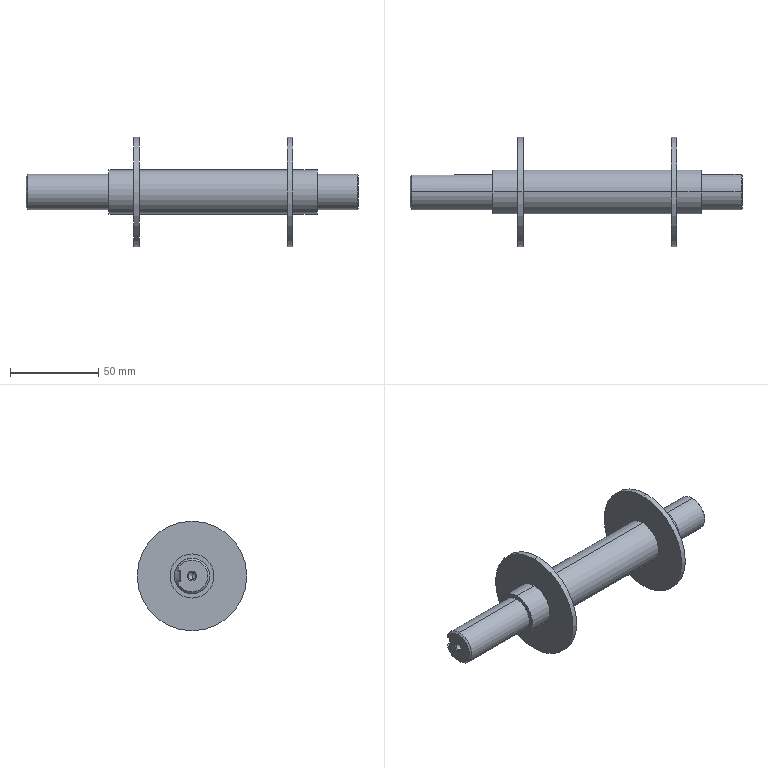Part | SolidWorks | features BaseBody 1 | 1 solid | 43 faces | box 188 x 62 x 62 mm | volume 94213 mm3 | cylinder 18 | cone 13 | plane 11 | spline 1 | commonest cylinder face diameters 25 x6 4.2 x4 20 x4 62 x4
STEP:
#1=CARTESIAN_POINT('',(-105.5,0.,-2.1));
#2=VERTEX_POINT('',#1);
#3=CARTESIAN_POINT('',(-105.5,0.,2.1));
#4=VERTEX_POINT('',#3);
#5=CARTESIAN_POINT('',(-105.5,0.,0.));
#6=DIRECTION('',(-1.,0.,0.));
#7=DIRECTION('',(0.,0.,1.));
#8=AXIS2_PLACEMENT_3D('',#5,#6,#7);
#9=CIRCLE('',#8,2.1);
#10=EDGE_CURVE('',#2,#4,#9,.T.);
#11=ORIENTED_EDGE('',*,*,#10,.F.);
#12=CARTESIAN_POINT('',(-106.,0.,-2.6));
#13=VERTEX_POINT('',#12);
#14=CARTESIAN_POINT('',(-105.5,0.,-2.1));
#15=DIRECTION('',(-0.7071,0.,-0.7071));
#16=VECTOR('',#15,1000.);
#17=LINE('',#14,#16);
#18=EDGE_CURVE('',#2,#13,#17,.T.);
#19=ORIENTED_EDGE('',*,*,#18,.T.);
#20=CARTESIAN_POINT('',(-106.,0.,2.6));
#21=VERTEX_POINT('',#20);
#22=CARTESIAN_POINT('',(-106.,0.,0.));
#23=DIRECTION('',(1.,0.,0.));
#24=DIRECTION('',(0.,0.,1.));
#25=AXIS2_PLACEMENT_3D('',#22,#23,#24);
#26=CIRCLE('',#25,2.6);
#27=EDGE_CURVE('',#21,#13,#26,.T.);
#28=ORIENTED_EDGE('',*,*,#27,.F.);
#29=CARTESIAN_POINT('',(-105.5,0.,2.1));
#30=DIRECTION('',(-0.7071,0.,0.7071));
#31=VECTOR('',#30,1000.);
#32=LINE('',#29,#31);
#33=EDGE_CURVE('',#4,#21,#32,.T.);
#34=ORIENTED_EDGE('',*,*,#33,.F.);
#35=EDGE_LOOP('',(#11,#19,#28,#34));
#36=FACE_OUTER_BOUND('',#35,.T.);
#37=CARTESIAN_POINT('',(-105.5,0.,0.));
#38=DIRECTION('',(-1.,0.,0.));
#39=DIRECTION('',(0.,0.,1.));
#40=AXIS2_PLACEMENT_3D('',#37,#38,#39);
#41=CONICAL_SURFACE('',#40,2.1,0.7854);
#42=ADVANCED_FACE('',(#36),#41,.F.);
#43=CARTESIAN_POINT('',(81.5,0.,2.1));
#44=VERTEX_POINT('',#43);
#45=CARTESIAN_POINT('',(81.5,0.,-2.1));
#46=VERTEX_POINT('',#45);
#47=CARTESIAN_POINT('',(81.5,0.,0.));
#48=DIRECTION('',(1.,0.,0.));
#49=DIRECTION('',(0.,0.,-1.));
#50=AXIS2_PLACEMENT_3D('',#47,#48,#49);
#51=CIRCLE('',#50,2.1);
#52=EDGE_CURVE('',#44,#46,#51,.T.);
#53=ORIENTED_EDGE('',*,*,#52,.F.);
#54=CARTESIAN_POINT('',(82.,0.,2.6));
#55=VERTEX_POINT('',#54);
#56=CARTESIAN_POINT('',(81.5,0.,2.1));
#57=DIRECTION('',(0.7071,0.,0.7071));
#58=VECTOR('',#57,1000.);
#59=LINE('',#56,#58);
#60=EDGE_CURVE('',#44,#55,#59,.T.);
#61=ORIENTED_EDGE('',*,*,#60,.T.);
#62=CARTESIAN_POINT('',(82.,0.,-2.6));
#63=VERTEX_POINT('',#62);
#64=CARTESIAN_POINT('',(82.,0.,0.));
#65=DIRECTION('',(-1.,0.,0.));
#66=DIRECTION('',(0.,0.,-1.));
#67=AXIS2_PLACEMENT_3D('',#64,#65,#66);
#68=CIRCLE('',#67,2.6);
#69=EDGE_CURVE('',#63,#55,#68,.T.);
#70=ORIENTED_EDGE('',*,*,#69,.F.);
#71=CARTESIAN_POINT('',(81.5,0.,-2.1));
#72=DIRECTION('',(0.7071,0.,-0.7071));
#73=VECTOR('',#72,1000.);
#74=LINE('',#71,#73);
#75=EDGE_CURVE('',#46,#63,#74,.T.);
#76=ORIENTED_EDGE('',*,*,#75,.F.);
#77=EDGE_LOOP('',(#53,#61,#70,#76));
#78=FACE_OUTER_BOUND('',#77,.T.);
#79=CARTESIAN_POINT('',(81.5,0.,0.));
#80=DIRECTION('',(1.,0.,0.));
#81=DIRECTION('',(0.,0.,-1.));
#82=AXIS2_PLACEMENT_3D('',#79,#80,#81);
#83=CONICAL_SURFACE('',#82,2.1,0.7854);
#84=ADVANCED_FACE('',(#78),#83,.F.);
#85=CARTESIAN_POINT('',(69.6,0.,2.1));
#86=VERTEX_POINT('',#85);
#87=CARTESIAN_POINT('',(69.6,0.,-2.1));
#88=VERTEX_POINT('',#87);
#89=CARTESIAN_POINT('',(69.6,0.,0.));
#90=DIRECTION('',(1.,0.,0.));
#91=DIRECTION('',(0.,0.,-1.));
#92=AXIS2_PLACEMENT_3D('',#89,#90,#91);
#93=CIRCLE('',#92,2.1);
#94=EDGE_CURVE('',#86,#88,#93,.T.);
#95=ORIENTED_EDGE('',*,*,#94,.F.);
#96=CARTESIAN_POINT('',(82.,0.,2.1));
#97=DIRECTION('',(1.,0.,0.));
#98=VECTOR('',#97,1000.);
#99=LINE('',#96,#98);
#100=EDGE_CURVE('',#86,#44,#99,.T.);
#101=ORIENTED_EDGE('',*,*,#100,.T.);
#102=ORIENTED_EDGE('',*,*,#52,.T.);
#103=CARTESIAN_POINT('',(82.,0.,-2.1));
#104=DIRECTION('',(1.,0.,0.));
#105=VECTOR('',#104,1000.);
#106=LINE('',#103,#105);
#107=EDGE_CURVE('',#88,#46,#106,.T.);
#108=ORIENTED_EDGE('',*,*,#107,.F.);
#109=EDGE_LOOP('',(#95,#101,#102,#108));
#110=FACE_OUTER_BOUND('',#109,.T.);
#111=CARTESIAN_POINT('',(82.,0.,0.));
#112=DIRECTION('',(1.,0.,0.));
#113=DIRECTION('',(0.,0.,-1.));
#114=AXIS2_PLACEMENT_3D('',#111,#112,#113);
#115=CYLINDRICAL_SURFACE('',#114,2.1);
#116=ADVANCED_FACE('',(#110),#115,.F.);
#117=CARTESIAN_POINT('',(68.338,0.,0.));
#118=VERTEX_POINT('',#117);
#119=CARTESIAN_POINT('',(69.6,0.,-2.1));
#120=DIRECTION('',(0.515,0.,-0.8572));
#121=VECTOR('',#120,1000.);
#122=LINE('',#119,#121);
#123=EDGE_CURVE('',#118,#88,#122,.T.);
#124=ORIENTED_EDGE('',*,*,#123,.F.);
#125=CARTESIAN_POINT('',(69.6,0.,2.1));
#126=DIRECTION('',(0.515,0.,0.8572));
#127=VECTOR('',#126,1000.);
#128=LINE('',#125,#127);
#129=EDGE_CURVE('',#118,#86,#128,.T.);
#130=ORIENTED_EDGE('',*,*,#129,.T.);
#131=ORIENTED_EDGE('',*,*,#94,.T.);
#132=EDGE_LOOP('',(#124,#130,#131));
#133=FACE_OUTER_BOUND('',#132,.T.);
#134=CARTESIAN_POINT('',(69.6,0.,0.));
#135=DIRECTION('',(1.,0.,0.));
#136=DIRECTION('',(0.,0.,-1.));
#137=AXIS2_PLACEMENT_3D('',#134,#135,#136);
#138=CONICAL_SURFACE('',#137,2.1,1.03);
#139=ADVANCED_FACE('',(#133),#138,.F.);
#140=CARTESIAN_POINT('',(-93.6,0.,-2.1));
#141=VERTEX_POINT('',#140);
#142=CARTESIAN_POINT('',(-93.6,0.,2.1));
#143=VERTEX_POINT('',#142);
#144=CARTESIAN_POINT('',(-93.6,0.,0.));
#145=DIRECTION('',(-1.,0.,0.));
#146=DIRECTION('',(0.,0.,1.));
#147=AXIS2_PLACEMENT_3D('',#144,#145,#146);
#148=CIRCLE('',#147,2.1);
#149=EDGE_CURVE('',#141,#143,#148,.T.);
#150=ORIENTED_EDGE('',*,*,#149,.F.);
#151=CARTESIAN_POINT('',(-106.,0.,-2.1));
#152=DIRECTION('',(-1.,0.,0.));
#153=VECTOR('',#152,1000.);
#154=LINE('',#151,#153);
#155=EDGE_CURVE('',#141,#2,#154,.T.);
#156=ORIENTED_EDGE('',*,*,#155,.T.);
#157=ORIENTED_EDGE('',*,*,#10,.T.);
#158=CARTESIAN_POINT('',(-106.,0.,2.1));
#159=DIRECTION('',(-1.,0.,0.));
#160=VECTOR('',#159,1000.);
#161=LINE('',#158,#160);
#162=EDGE_CURVE('',#143,#4,#161,.T.);
#163=ORIENTED_EDGE('',*,*,#162,.F.);
#164=EDGE_LOOP('',(#150,#156,#157,#163));
#165=FACE_OUTER_BOUND('',#164,.T.);
#166=CARTESIAN_POINT('',(-106.,0.,0.));
#167=DIRECTION('',(-1.,0.,0.));
#168=DIRECTION('',(0.,0.,1.));
#169=AXIS2_PLACEMENT_3D('',#166,#167,#168);
#170=CYLINDRICAL_SURFACE('',#169,2.1);
#171=ADVANCED_FACE('',(#165),#170,.F.);
#172=CARTESIAN_POINT('',(-92.338,0.,0.));
#173=VERTEX_POINT('',#172);
#174=CARTESIAN_POINT('',(-93.6,0.,2.1));
#175=DIRECTION('',(-0.515,0.,0.8572));
#176=VECTOR('',#175,1000.);
#177=LINE('',#174,#176);
#178=EDGE_CURVE('',#173,#143,#177,.T.);
#179=ORIENTED_EDGE('',*,*,#178,.F.);
#180=CARTESIAN_POINT('',(-93.6,0.,-2.1));
#181=DIRECTION('',(-0.515,0.,-0.8572));
#182=VECTOR('',#181,1000.);
#183=LINE('',#180,#182);
#184=EDGE_CURVE('',#173,#141,#183,.T.);
#185=ORIENTED_EDGE('',*,*,#184,.T.);
#186=ORIENTED_EDGE('',*,*,#149,.T.);
#187=EDGE_LOOP('',(#179,#185,#186));
#188=FACE_OUTER_BOUND('',#187,.T.);
#189=CARTESIAN_POINT('',(-93.6,0.,0.));
#190=DIRECTION('',(-1.,0.,0.));
#191=DIRECTION('',(0.,0.,1.));
#192=AXIS2_PLACEMENT_3D('',#189,#190,#191);
#193=CONICAL_SURFACE('',#192,2.1,1.03);
#194=ADVANCED_FACE('',(#188),#193,.F.);
#195=CARTESIAN_POINT('',(82.,0.,-9.5));
#196=VERTEX_POINT('',#195);
#197=CARTESIAN_POINT('',(82.,0.,9.5));
#198=VERTEX_POINT('',#197);
#199=CARTESIAN_POINT('',(82.,0.,0.));
#200=DIRECTION('',(1.,0.,0.));
#201=DIRECTION('',(0.,0.,-1.));
#202=AXIS2_PLACEMENT_3D('',#199,#200,#201);
#203=CIRCLE('',#202,9.5);
#204=EDGE_CURVE('',#196,#198,#203,.T.);
#205=ORIENTED_EDGE('',*,*,#204,.F.);
#206=CARTESIAN_POINT('',(81.5,0.,-10.));
#207=VERTEX_POINT('',#206);
#208=CARTESIAN_POINT('',(82.,0.,-9.5));
#209=DIRECTION('',(-0.7071,0.,-0.7071));
#210=VECTOR('',#209,1000.);
#211=LINE('',#208,#210);
#212=EDGE_CURVE('',#196,#207,#211,.T.);
#213=ORIENTED_EDGE('',*,*,#212,.T.);
#214=CARTESIAN_POINT('',(81.5,0.,10.));
#215=VERTEX_POINT('',#214);
#216=CARTESIAN_POINT('',(81.5,0.,0.));
#217=DIRECTION('',(-1.,0.,0.));
#218=DIRECTION('',(0.,0.,-1.));
#219=AXIS2_PLACEMENT_3D('',#216,#217,#218);
#220=CIRCLE('',#219,10.);
#221=EDGE_CURVE('',#215,#207,#220,.T.);
#222=ORIENTED_EDGE('',*,*,#221,.F.);
#223=CARTESIAN_POINT('',(82.,0.,9.5));
#224=DIRECTION('',(-0.7071,0.,0.7071));
#225=VECTOR('',#224,1000.);
#226=LINE('',#223,#225);
#227=EDGE_CURVE('',#198,#215,#226,.T.);
#228=ORIENTED_EDGE('',*,*,#227,.F.);
#229=EDGE_LOOP('',(#205,#213,#222,#228));
#230=FACE_OUTER_BOUND('',#229,.T.);
#231=CARTESIAN_POINT('',(82.,0.,0.));
#232=DIRECTION('',(-1.,0.,0.));
#233=DIRECTION('',(0.,0.,1.));
#234=AXIS2_PLACEMENT_3D('',#231,#232,#233);
#235=CONICAL_SURFACE('',#234,9.5,0.7854);
#236=ADVANCED_FACE('',(#230),#235,.T.);
#237=ORIENTED_EDGE('',*,*,#221,.T.);
#238=CARTESIAN_POINT('',(59.,0.,-10.));
#239=VERTEX_POINT('',#238);
#240=CARTESIAN_POINT('',(82.,0.,-10.));
#241=DIRECTION('',(-1.,0.,0.));
#242=VECTOR('',#241,1000.);
#243=LINE('',#240,#242);
#244=EDGE_CURVE('',#207,#239,#243,.T.);
#245=ORIENTED_EDGE('',*,*,#244,.T.);
#246=CARTESIAN_POINT('',(59.,0.,10.));
#247=VERTEX_POINT('',#246);
#248=CARTESIAN_POINT('',(59.,0.,0.));
#249=DIRECTION('',(1.,0.,0.));
#250=DIRECTION('',(0.,0.,-1.));
#251=AXIS2_PLACEMENT_3D('',#248,#249,#250);
#252=CIRCLE('',#251,10.);
#253=EDGE_CURVE('',#239,#247,#252,.T.);
#254=ORIENTED_EDGE('',*,*,#253,.T.);
#255=CARTESIAN_POINT('',(82.,0.,10.));
#256=DIRECTION('',(-1.,0.,0.));
#257=VECTOR('',#256,1000.);
#258=LINE('',#255,#257);
#259=EDGE_CURVE('',#215,#247,#258,.T.);
#260=ORIENTED_EDGE('',*,*,#259,.F.);
#261=EDGE_LOOP('',(#237,#245,#254,#260));
#262=FACE_OUTER_BOUND('',#261,.T.);
#263=CARTESIAN_POINT('',(82.,0.,0.));
#264=DIRECTION('',(-1.,0.,0.));
#265=DIRECTION('',(0.,0.,1.));
#266=AXIS2_PLACEMENT_3D('',#263,#264,#265);
#267=CYLINDRICAL_SURFACE('',#266,10.);
#268=ADVANCED_FACE('',(#262),#267,.T.);
#269=CARTESIAN_POINT('',(-106.,0.,9.));
#270=VERTEX_POINT('',#269);
#271=CARTESIAN_POINT('',(-106.,8.485,3.));
#272=VERTEX_POINT('',#271);
#273=CARTESIAN_POINT('',(-106.,0.,0.));
#274=DIRECTION('',(-1.,0.,0.));
#275=DIRECTION('',(0.,0.,1.));
#276=AXIS2_PLACEMENT_3D('',#273,#274,#275);
#277=CIRCLE('',#276,9.);
#278=EDGE_CURVE('',#270,#272,#277,.T.);
#279=ORIENTED_EDGE('',*,*,#278,.F.);
#280=CARTESIAN_POINT('',(-105.,0.,10.));
#281=VERTEX_POINT('',#280);
#282=CARTESIAN_POINT('',(-106.,0.,9.));
#283=DIRECTION('',(0.7071,0.,0.7071));
#284=VECTOR('',#283,1000.);
#285=LINE('',#282,#284);
#286=EDGE_CURVE('',#270,#281,#285,.T.);
#287=ORIENTED_EDGE('',*,*,#286,.T.);
#288=CARTESIAN_POINT('',(-105.,9.539,3.));
#289=VERTEX_POINT('',#288);
#290=CARTESIAN_POINT('',(-105.,0.,0.));
#291=DIRECTION('',(1.,0.,0.));
#292=DIRECTION('',(0.,0.,1.));
#293=AXIS2_PLACEMENT_3D('',#290,#291,#292);
#294=CIRCLE('',#293,10.);
#295=EDGE_CURVE('',#289,#281,#294,.T.);
#296=ORIENTED_EDGE('',*,*,#295,.F.);
#297=CARTESIAN_POINT('',(-106.,8.485,3.));
#298=CARTESIAN_POINT('',(-105.668,8.838,3.));
#299=CARTESIAN_POINT('',(-105.334,9.189,3.));
#300=CARTESIAN_POINT('',(-105.,9.539,3.));
#301=B_SPLINE_CURVE_WITH_KNOTS('',3,(#297,#298,#299,#300),.UNSPECIFIED.,.F.,.F.,(4,4),(0.006491,0.007944),.UNSPECIFIED.);
#302=EDGE_CURVE('',#272,#289,#301,.T.);
#303=ORIENTED_EDGE('',*,*,#302,.F.);
#304=EDGE_LOOP('',(#279,#287,#296,#303));
#305=FACE_OUTER_BOUND('',#304,.T.);
#306=CARTESIAN_POINT('',(-106.,0.,0.));
#307=DIRECTION('',(1.,0.,0.));
#308=DIRECTION('',(0.,0.,-1.));
#309=AXIS2_PLACEMENT_3D('',#306,#307,#308);
#310=CONICAL_SURFACE('',#309,9.,0.7854);
#311=ADVANCED_FACE('',(#305),#310,.T.);
#312=ORIENTED_EDGE('',*,*,#286,.F.);
#313=CARTESIAN_POINT('',(-106.,0.,-9.));
#314=VERTEX_POINT('',#313);
#315=CARTESIAN_POINT('',(-106.,0.,0.));
#316=DIRECTION('',(-1.,0.,0.));
#317=DIRECTION('',(0.,0.,1.));
#318=AXIS2_PLACEMENT_3D('',#315,#316,#317);
#319=CIRCLE('',#318,9.);
#320=EDGE_CURVE('',#314,#270,#319,.T.);
#321=ORIENTED_EDGE('',*,*,#320,.F.);
#322=CARTESIAN_POINT('',(-105.,0.,-10.));
#323=VERTEX_POINT('',#322);
#324=CARTESIAN_POINT('',(-106.,0.,-9.));
#325=DIRECTION('',(0.7071,0.,-0.7071));
#326=VECTOR('',#325,1000.);
#327=LINE('',#324,#326);
#328=EDGE_CURVE('',#314,#323,#327,.T.);
#329=ORIENTED_EDGE('',*,*,#328,.T.);
#330=CARTESIAN_POINT('',(-105.,0.,0.));
#331=DIRECTION('',(1.,0.,0.));
#332=DIRECTION('',(0.,0.,1.));
#333=AXIS2_PLACEMENT_3D('',#330,#331,#332);
#334=CIRCLE('',#333,10.);
#335=EDGE_CURVE('',#281,#323,#334,.T.);
#336=ORIENTED_EDGE('',*,*,#335,.F.);
#337=EDGE_LOOP('',(#312,#321,#329,#336));
#338=FACE_OUTER_BOUND('',#337,.T.);
#339=CARTESIAN_POINT('',(-106.,0.,0.));
#340=DIRECTION('',(1.,0.,0.));
#341=DIRECTION('',(0.,0.,-1.));
#342=AXIS2_PLACEMENT_3D('',#339,#340,#341);
#343=CONICAL_SURFACE('',#342,9.,0.7854);
#344=ADVANCED_FACE('',(#338),#343,.T.);
#345=ORIENTED_EDGE('',*,*,#295,.T.);
#346=CARTESIAN_POINT('',(-59.,0.,10.));
#347=VERTEX_POINT('',#346);
#348=CARTESIAN_POINT('',(-106.,0.,10.));
#349=DIRECTION('',(1.,0.,0.));
#350=VECTOR('',#349,1000.);
#351=LINE('',#348,#350);
#352=EDGE_CURVE('',#281,#347,#351,.T.);
#353=ORIENTED_EDGE('',*,*,#352,.T.);
#354=CARTESIAN_POINT('',(-59.,0.,-10.));
#355=VERTEX_POINT('',#354);
#356=CARTESIAN_POINT('',(-59.,0.,0.));
#357=DIRECTION('',(-1.,0.,0.));
#358=DIRECTION('',(0.,0.,1.));
#359=AXIS2_PLACEMENT_3D('',#356,#357,#358);
#360=CIRCLE('',#359,10.);
#361=EDGE_CURVE('',#347,#355,#360,.T.);
#362=ORIENTED_EDGE('',*,*,#361,.T.);
#363=CARTESIAN_POINT('',(-106.,0.,-10.));
#364=DIRECTION('',(1.,0.,0.));
#365=VECTOR('',#364,1000.);
#366=LINE('',#363,#365);
#367=EDGE_CURVE('',#323,#355,#366,.T.);
#368=ORIENTED_EDGE('',*,*,#367,.F.);
#369=CARTESIAN_POINT('',(-105.,9.539,-3.));
#370=VERTEX_POINT('',#369);
#371=CARTESIAN_POINT('',(-105.,0.,0.));
#372=DIRECTION('',(1.,0.,0.));
#373=DIRECTION('',(0.,0.,1.));
#374=AXIS2_PLACEMENT_3D('',#371,#372,#373);
#375=CIRCLE('',#374,10.);
#376=EDGE_CURVE('',#323,#370,#375,.T.);
#377=ORIENTED_EDGE('',*,*,#376,.T.);
#378=CARTESIAN_POINT('',(-81.,9.539,-3.));
#379=VERTEX_POINT('',#378);
#380=CARTESIAN_POINT('',(-106.,9.539,-3.));
#381=DIRECTION('',(1.,0.,0.));
#382=VECTOR('',#381,1000.);
#383=LINE('',#380,#382);
#384=EDGE_CURVE('',#370,#379,#383,.T.);
#385=ORIENTED_EDGE('',*,*,#384,.T.);
#386=CARTESIAN_POINT('',(-81.,9.539,3.));
#387=VERTEX_POINT('',#386);
#388=CARTESIAN_POINT('',(-81.,9.539,3.));
#389=CARTESIAN_POINT('',(-81.,9.692,2.514));
#390=CARTESIAN_POINT('',(-81.,9.807,2.019));
#391=CARTESIAN_POINT('',(-81.,9.962,1.011));
#392=CARTESIAN_POINT('',(-81.,10.,0.5036));
#393=CARTESIAN_POINT('',(-81.,10.,-0.5143));
#394=CARTESIAN_POINT('',(-81.,9.96,-1.022));
#395=CARTESIAN_POINT('',(-81.,9.807,-2.021));
#396=CARTESIAN_POINT('',(-81.,9.692,-2.514));
#397=CARTESIAN_POINT('',(-81.,9.539,-3.));
#398=B_SPLINE_CURVE_WITH_KNOTS('',3,(#388,#389,#390,#391,#392,#393,#394,#395,#396,#397),.UNSPECIFIED.,.F.,.F.,(4,2,2,2,4),(0.,0.001525,0.003049,0.004574,0.006098),.UNSPECIFIED.);
#399=EDGE_CURVE('',#387,#379,#398,.T.);
#400=ORIENTED_EDGE('',*,*,#399,.F.);
#401=CARTESIAN_POINT('',(-106.,9.539,3.));
#402=DIRECTION('',(-1.,0.,0.));
#403=VECTOR('',#402,1000.);
#404=LINE('',#401,#403);
#405=EDGE_CURVE('',#387,#289,#404,.T.);
#406=ORIENTED_EDGE('',*,*,#405,.T.);
#407=EDGE_LOOP('',(#345,#353,#362,#368,#377,#385,#400,#406));
#408=FACE_OUTER_BOUND('',#407,.T.);
#409=CARTESIAN_POINT('',(-106.,0.,0.));
#410=DIRECTION('',(1.,0.,0.));
#411=DIRECTION('',(0.,0.,-1.));
#412=AXIS2_PLACEMENT_3D('',#409,#410,#411);
#413=CYLINDRICAL_SURFACE('',#412,10.);
#414=ADVANCED_FACE('',(#408),#413,.T.);
#415=CARTESIAN_POINT('',(59.,0.,12.5));
#416=VERTEX_POINT('',#415);
#417=CARTESIAN_POINT('',(59.,0.,-12.5));
#418=VERTEX_POINT('',#417);
#419=CARTESIAN_POINT('',(59.,0.,0.));
#420=DIRECTION('',(-1.,0.,0.));
#421=DIRECTION('',(0.,0.,1.));
#422=AXIS2_PLACEMENT_3D('',#419,#420,#421);
#423=CIRCLE('',#422,12.5);
#424=EDGE_CURVE('',#416,#418,#423,.T.);
#425=ORIENTED_EDGE('',*,*,#424,.T.);
#426=CARTESIAN_POINT('',(45.,0.,-12.5));
#427=VERTEX_POINT('',#426);
#428=CARTESIAN_POINT('',(-45.,0.,-12.5));
#429=DIRECTION('',(-1.,0.,0.));
#430=VECTOR('',#429,1000.);
#431=LINE('',#428,#430);
#432=EDGE_CURVE('',#418,#427,#431,.T.);
#433=ORIENTED_EDGE('',*,*,#432,.T.);
#434=CARTESIAN_POINT('',(45.,0.,12.5));
#435=VERTEX_POINT('',#434);
#436=CARTESIAN_POINT('',(45.,0.,0.));
#437=DIRECTION('',(-1.,0.,0.));
#438=DIRECTION('',(0.,0.,1.));
#439=AXIS2_PLACEMENT_3D('',#436,#437,#438);
#440=CIRCLE('',#439,12.5);
#441=EDGE_CURVE('',#435,#427,#440,.T.);
#442=ORIENTED_EDGE('',*,*,#441,.F.);
#443=CARTESIAN_POINT('',(-45.,0.,12.5));
#444=DIRECTION('',(-1.,0.,0.));
#445=VECTOR('',#444,1000.);
#446=LINE('',#443,#445);
#447=EDGE_CURVE('',#416,#435,#446,.T.);
#448=ORIENTED_EDGE('',*,*,#447,.F.);
#449=EDGE_LOOP('',(#425,#433,#442,#448));
#450=FACE_OUTER_BOUND('',#449,.T.);
#451=CARTESIAN_POINT('',(-45.,0.,0.));
#452=DIRECTION('',(-1.,0.,0.));
#453=DIRECTION('',(0.,0.,1.));
#454=AXIS2_PLACEMENT_3D('',#451,#452,#453);
#455=CYLINDRICAL_SURFACE('',#454,12.5);
#456=ADVANCED_FACE('',(#450),#455,.T.);
#457=CARTESIAN_POINT('',(45.,0.,31.));
#458=VERTEX_POINT('',#457);
#459=CARTESIAN_POINT('',(45.,0.,-31.));
#460=VERTEX_POINT('',#459);
#461=CARTESIAN_POINT('',(45.,0.,0.));
#462=DIRECTION('',(-1.,0.,0.));
#463=DIRECTION('',(0.,0.,1.));
#464=AXIS2_PLACEMENT_3D('',#461,#462,#463);
#465=CIRCLE('',#464,31.);
#466=EDGE_CURVE('',#458,#460,#465,.T.);
#467=ORIENTED_EDGE('',*,*,#466,.T.);
#468=CARTESIAN_POINT('',(42.,0.,-31.));
#469=VERTEX_POINT('',#468);
#470=CARTESIAN_POINT('',(-45.,0.,-31.));
#471=DIRECTION('',(-1.,0.,0.));
#472=VECTOR('',#471,1000.);
#473=LINE('',#470,#472);
#474=EDGE_CURVE('',#460,#469,#473,.T.);
#475=ORIENTED_EDGE('',*,*,#474,.T.);
#476=CARTESIAN_POINT('',(42.,0.,31.));
#477=VERTEX_POINT('',#476);
#478=CARTESIAN_POINT('',(42.,0.,0.));
#479=DIRECTION('',(1.,0.,0.));
#480=DIRECTION('',(0.,0.,-1.));
#481=AXIS2_PLACEMENT_3D('',#478,#479,#480);
#482=CIRCLE('',#481,31.);
#483=EDGE_CURVE('',#469,#477,#482,.T.);
#484=ORIENTED_EDGE('',*,*,#483,.T.);
#485=CARTESIAN_POINT('',(-45.,0.,31.));
#486=DIRECTION('',(-1.,0.,0.));
#487=VECTOR('',#486,1000.);
#488=LINE('',#485,#487);
#489=EDGE_CURVE('',#458,#477,#488,.T.);
#490=ORIENTED_EDGE('',*,*,#489,.F.);
#491=EDGE_LOOP('',(#467,#475,#484,#490));
#492=FACE_OUTER_BOUND('',#491,.T.);
#493=CARTESIAN_POINT('',(-45.,0.,0.));
#494=DIRECTION('',(-1.,0.,0.));
#495=DIRECTION('',(0.,0.,1.));
#496=AXIS2_PLACEMENT_3D('',#493,#494,#495);
#497=CYLINDRICAL_SURFACE('',#496,31.);
#498=ADVANCED_FACE('',(#492),#497,.T.);
#499=CARTESIAN_POINT('',(-45.,0.,12.5));
#500=VERTEX_POINT('',#499);
#501=CARTESIAN_POINT('',(-45.,0.,-12.5));
#502=VERTEX_POINT('',#501);
#503=CARTESIAN_POINT('',(-45.,0.,0.));
#504=DIRECTION('',(-1.,0.,0.));
#505=DIRECTION('',(0.,0.,-1.));
#506=AXIS2_PLACEMENT_3D('',#503,#504,#505);
#507=CIRCLE('',#506,12.5);
#508=EDGE_CURVE('',#500,#502,#507,.T.);
#509=ORIENTED_EDGE('',*,*,#508,.T.);
#510=CARTESIAN_POINT('',(-59.,0.,-12.5));
#511=VERTEX_POINT('',#510);
#512=CARTESIAN_POINT('',(-45.,0.,-12.5));
#513=DIRECTION('',(-1.,0.,0.));
#514=VECTOR('',#513,1000.);
#515=LINE('',#512,#514);
#516=EDGE_CURVE('',#502,#511,#515,.T.);
#517=ORIENTED_EDGE('',*,*,#516,.T.);
#518=CARTESIAN_POINT('',(-59.,0.,12.5));
#519=VERTEX_POINT('',#518);
#520=CARTESIAN_POINT('',(-59.,0.,0.));
#521=DIRECTION('',(-1.,0.,0.));
#522=DIRECTION('',(0.,0.,1.));
#523=AXIS2_PLACEMENT_3D('',#520,#521,#522);
#524=CIRCLE('',#523,12.5);
#525=EDGE_CURVE('',#519,#511,#524,.T.);
#526=ORIENTED_EDGE('',*,*,#525,.F.);
#527=CARTESIAN_POINT('',(-45.,0.,12.5));
#528=DIRECTION('',(-1.,0.,0.));
#529=VECTOR('',#528,1000.);
#530=LINE('',#527,#529);
#531=EDGE_CURVE('',#500,#519,#530,.T.);
#532=ORIENTED_EDGE('',*,*,#531,.F.);
#533=EDGE_LOOP('',(#509,#517,#526,#532));
#534=FACE_OUTER_BOUND('',#533,.T.);
#535=CARTESIAN_POINT('',(-45.,0.,0.));
#536=DIRECTION('',(-1.,0.,0.));
#537=DIRECTION('',(0.,0.,1.));
#538=AXIS2_PLACEMENT_3D('',#535,#536,#537);
#539=CYLINDRICAL_SURFACE('',#538,12.5);
#540=ADVANCED_FACE('',(#534),#539,.T.);
#541=CARTESIAN_POINT('',(-42.,0.,-31.));
#542=VERTEX_POINT('',#541);
#543=CARTESIAN_POINT('',(-42.,0.,31.));
#544=VERTEX_POINT('',#543);
#545=CARTESIAN_POINT('',(-42.,0.,0.));
#546=DIRECTION('',(1.,0.,0.));
#547=DIRECTION('',(0.,0.,-1.));
#548=AXIS2_PLACEMENT_3D('',#545,#546,#547);
#549=CIRCLE('',#548,31.);
#550=EDGE_CURVE('',#542,#544,#549,.T.);
#551=ORIENTED_EDGE('',*,*,#550,.F.);
#552=CARTESIAN_POINT('',(-45.,0.,-31.));
#553=VERTEX_POINT('',#552);
#554=CARTESIAN_POINT('',(-45.,0.,-31.));
#555=DIRECTION('',(-1.,0.,0.));
#556=VECTOR('',#555,1000.);
#557=LINE('',#554,#556);
#558=EDGE_CURVE('',#542,#553,#557,.T.);
#559=ORIENTED_EDGE('',*,*,#558,.T.);
#560=CARTESIAN_POINT('',(-45.,0.,31.));
#561=VERTEX_POINT('',#560);
#562=CARTESIAN_POINT('',(-45.,0.,0.));
#563=DIRECTION('',(-1.,0.,0.));
#564=DIRECTION('',(0.,0.,1.));
#565=AXIS2_PLACEMENT_3D('',#562,#563,#564);
#566=CIRCLE('',#565,31.);
#567=EDGE_CURVE('',#561,#553,#566,.T.);
#568=ORIENTED_EDGE('',*,*,#567,.F.);
#569=CARTESIAN_POINT('',(-45.,0.,31.));
#570=DIRECTION('',(-1.,0.,0.));
#571=VECTOR('',#570,1000.);
#572=LINE('',#569,#571);
#573=EDGE_CURVE('',#544,#561,#572,.T.);
#574=ORIENTED_EDGE('',*,*,#573,.F.);
#575=EDGE_LOOP('',(#551,#559,#568,#574));
#576=FACE_OUTER_BOUND('',#575,.T.);
#577=CARTESIAN_POINT('',(-45.,0.,0.));
#578=DIRECTION('',(-1.,0.,0.));
#579=DIRECTION('',(0.,0.,1.));
#580=AXIS2_PLACEMENT_3D('',#577,#578,#579);
#581=CYLINDRICAL_SURFACE('',#580,31.);
#582=ADVANCED_FACE('',(#576),#581,.T.);
#583=CARTESIAN_POINT('',(42.,0.,-12.5));
#584=VERTEX_POINT('',#583);
#585=CARTESIAN_POINT('',(42.,0.,12.5));
#586=VERTEX_POINT('',#585);
#587=CARTESIAN_POINT('',(42.,0.,0.));
#588=DIRECTION('',(1.,0.,0.));
#589=DIRECTION('',(0.,0.,-1.));
#590=AXIS2_PLACEMENT_3D('',#587,#588,#589);
#591=CIRCLE('',#590,12.5);
#592=EDGE_CURVE('',#584,#586,#591,.T.);
#593=ORIENTED_EDGE('',*,*,#592,.F.);
#594=CARTESIAN_POINT('',(-42.,0.,-12.5));
#595=VERTEX_POINT('',#594);
#596=CARTESIAN_POINT('',(-45.,0.,-12.5));
#597=DIRECTION('',(-1.,0.,0.));
#598=VECTOR('',#597,1000.);
#599=LINE('',#596,#598);
#600=EDGE_CURVE('',#584,#595,#599,.T.);
#601=ORIENTED_EDGE('',*,*,#600,.T.);
#602=CARTESIAN_POINT('',(-42.,0.,12.5));
#603=VERTEX_POINT('',#602);
#604=CARTESIAN_POINT('',(-42.,0.,0.));
#605=DIRECTION('',(1.,0.,0.));
#606=DIRECTION('',(0.,0.,-1.));
#607=AXIS2_PLACEMENT_3D('',#604,#605,#606);
#608=CIRCLE('',#607,12.5);
#609=EDGE_CURVE('',#595,#603,#608,.T.);
#610=ORIENTED_EDGE('',*,*,#609,.T.);
#611=CARTESIAN_POINT('',(-45.,0.,12.5));
#612=DIRECTION('',(-1.,0.,0.));
#613=VECTOR('',#612,1000.);
#614=LINE('',#611,#613);
#615=EDGE_CURVE('',#586,#603,#614,.T.);
#616=ORIENTED_EDGE('',*,*,#615,.F.);
#617=EDGE_LOOP('',(#593,#601,#610,#616));
#618=FACE_OUTER_BOUND('',#617,.T.);
#619=CARTESIAN_POINT('',(-45.,0.,0.));
#620=DIRECTION('',(-1.,0.,0.));
#621=DIRECTION('',(0.,0.,1.));
#622=AXIS2_PLACEMENT_3D('',#619,#620,#621);
#623=CYLINDRICAL_SURFACE('',#622,12.5);
#624=ADVANCED_FACE('',(#618),#623,.T.);
#625=CARTESIAN_POINT('',(-85.631,6.5,-3.));
#626=VERTEX_POINT('',#625);
#627=CARTESIAN_POINT('',(-85.631,6.5,-3.));
#628=CARTESIAN_POINT('',(-85.138,6.5,-3.));
#629=CARTESIAN_POINT('',(-84.657,6.571,-3.));
#630=CARTESIAN_POINT('',(-83.954,6.78,-3.));
#631=CARTESIAN_POINT('',(-83.722,6.868,-3.));
#632=CARTESIAN_POINT('',(-83.28,7.073,-3.));
#633=CARTESIAN_POINT('',(-83.068,7.191,-3.));
#634=CARTESIAN_POINT('',(-82.66,7.458,-3.));
#635=CARTESIAN_POINT('',(-82.463,7.608,-3.));
#636=CARTESIAN_POINT('',(-82.097,7.933,-3.));
#637=CARTESIAN_POINT('',(-81.927,8.107,-3.));
#638=CARTESIAN_POINT('',(-81.457,8.664,-3.));
#639=CARTESIAN_POINT('',(-81.195,9.087,-3.));
#640=CARTESIAN_POINT('',(-81.,9.539,-3.));
#641=B_SPLINE_CURVE_WITH_KNOTS('',3,(#627,#628,#629,#630,#631,#632,#633,#634,#635,#636,#637,#638,#639,#640),.UNSPECIFIED.,.F.,.F.,(4,2,2,2,2,2,4),(0.,0.001458,0.002187,0.002916,0.003645,0.004373,0.005831),.UNSPECIFIED.);
#642=EDGE_CURVE('',#626,#379,#641,.T.);
#643=ORIENTED_EDGE('',*,*,#642,.F.);
#644=CARTESIAN_POINT('',(-85.631,6.5,3.));
#645=VERTEX_POINT('',#644);
#646=CARTESIAN_POINT('',(-85.631,6.5,3.));
#647=CARTESIAN_POINT('',(-85.734,6.5,2.002));
#648=CARTESIAN_POINT('',(-85.77,6.5,0.9991));
#649=CARTESIAN_POINT('',(-85.77,6.5,-1.002));
#650=CARTESIAN_POINT('',(-85.734,6.5,-2.002));
#651=CARTESIAN_POINT('',(-85.631,6.5,-3.));
#652=B_SPLINE_CURVE_WITH_KNOTS('',3,(#646,#647,#648,#649,#650,#651),.UNSPECIFIED.,.F.,.F.,(4,2,4),(0.,0.003008,0.006016),.UNSPECIFIED.);
#653=EDGE_CURVE('',#645,#626,#652,.T.);
#654=ORIENTED_EDGE('',*,*,#653,.F.);
#655=CARTESIAN_POINT('',(-81.,9.539,3.));
#656=CARTESIAN_POINT('',(-81.195,9.087,3.));
#657=CARTESIAN_POINT('',(-81.451,8.673,3.));
#658=CARTESIAN_POINT('',(-81.923,8.111,3.));
#659=CARTESIAN_POINT('',(-82.096,7.934,3.));
#660=CARTESIAN_POINT('',(-82.46,7.611,3.));
#661=CARTESIAN_POINT('',(-82.653,7.463,3.));
#662=CARTESIAN_POINT('',(-83.061,7.195,3.));
#663=CARTESIAN_POINT('',(-83.277,7.075,3.));
#664=CARTESIAN_POINT('',(-83.72,6.869,3.));
#665=CARTESIAN_POINT('',(-83.948,6.782,3.));
#666=CARTESIAN_POINT('',(-84.646,6.573,3.));
#667=CARTESIAN_POINT('',(-85.138,6.5,3.));
#668=CARTESIAN_POINT('',(-85.631,6.5,3.));
#669=B_SPLINE_CURVE_WITH_KNOTS('',3,(#655,#656,#657,#658,#659,#660,#661,#662,#663,#664,#665,#666,#667,#668),.UNSPECIFIED.,.F.,.F.,(4,2,2,2,2,2,4),(0.,0.001458,0.002187,0.002915,0.003644,0.004373,0.005831),.UNSPECIFIED.);
#670=EDGE_CURVE('',#387,#645,#669,.T.);
#671=ORIENTED_EDGE('',*,*,#670,.F.);
#672=ORIENTED_EDGE('',*,*,#399,.T.);
#673=EDGE_LOOP('',(#643,#654,#671,#672));
#674=FACE_OUTER_BOUND('',#673,.T.);
#675=CARTESIAN_POINT('',(-81.,9.529,-3.032));
#676=CARTESIAN_POINT('',(-82.287,6.5,-3.21));
#677=CARTESIAN_POINT('',(-85.552,6.5,-3.66));
#678=CARTESIAN_POINT('',(-81.,9.674,-2.577));
#679=CARTESIAN_POINT('',(-82.242,6.5,-2.697));
#680=CARTESIAN_POINT('',(-85.636,6.5,-3.054));
#681=CARTESIAN_POINT('',(-81.,9.793,-2.088));
#682=CARTESIAN_POINT('',(-82.194,6.5,-2.175));
#683=CARTESIAN_POINT('',(-85.688,6.5,-2.447));
#684=CARTESIAN_POINT('',(-81.,9.956,-1.069));
#685=CARTESIAN_POINT('',(-82.122,6.5,-1.102));
#686=CARTESIAN_POINT('',(-85.755,6.5,-1.229));
#687=CARTESIAN_POINT('',(-81.,10.,-0.5385));
#688=CARTESIAN_POINT('',(-82.101,6.5,-0.5571));
#689=CARTESIAN_POINT('',(-85.77,6.5,-0.6192));
#690=CARTESIAN_POINT('',(-81.,10.,0.5242));
#691=CARTESIAN_POINT('',(-82.101,6.5,0.5423));
#692=CARTESIAN_POINT('',(-85.77,6.5,0.6028));
#693=CARTESIAN_POINT('',(-81.,9.958,1.056));
#694=CARTESIAN_POINT('',(-82.122,6.5,1.089));
#695=CARTESIAN_POINT('',(-85.755,6.5,1.215));
#696=CARTESIAN_POINT('',(-81.,9.794,2.084));
#697=CARTESIAN_POINT('',(-82.193,6.5,2.17));
#698=CARTESIAN_POINT('',(-85.688,6.5,2.441));
#699=CARTESIAN_POINT('',(-81.,9.674,2.576));
#700=CARTESIAN_POINT('',(-82.242,6.5,2.696));
#701=CARTESIAN_POINT('',(-85.636,6.5,3.052));
#702=CARTESIAN_POINT('',(-81.,9.529,3.033));
#703=CARTESIAN_POINT('',(-82.287,6.5,3.21));
#704=CARTESIAN_POINT('',(-85.552,6.5,3.66));
#705=(BOUNDED_SURFACE()B_SPLINE_SURFACE(3,2,((#675,#676,#677),(#678,#679,#680),(#681,#682,#683),(#684,#685,#686),(#687,#688,#689),(#690,#691,#692),(#693,#694,#695),(#696,#697,#698),(#699,#700,#701),(#702,#703,#704)),.UNSPECIFIED.,.F.,.F.,.T.)B_SPLINE_SURFACE_WITH_KNOTS((4,2,2,2,4),(3,3),(0.008171,0.01002,0.01187,0.01371,0.01556),(0.,1.),.UNSPECIFIED.)GEOMETRIC_REPRESENTATION_ITEM()RATIONAL_B_SPLINE_SURFACE(((1.,0.8349,1.),(1.,0.8262,1.),(1.,0.819,1.),(1.,0.809,1.),(1.,0.8062,1.),(1.,0.8062,1.),(1.,0.8089,1.),(1.,0.8189,1.),(1.,0.8262,1.),(1.,0.8349,1.)))REPRESENTATION_ITEM('')SURFACE());
#706=ADVANCED_FACE('',(#674),#705,.F.);
#707=CARTESIAN_POINT('',(-106.,6.5,3.));
#708=VERTEX_POINT('',#707);
#709=CARTESIAN_POINT('',(-81.,6.5,3.));
#710=DIRECTION('',(-1.,0.,0.));
#711=VECTOR('',#710,1000.);
#712=LINE('',#709,#711);
#713=EDGE_CURVE('',#645,#708,#712,.T.);
#714=ORIENTED_EDGE('',*,*,#713,.F.);
#715=ORIENTED_EDGE('',*,*,#653,.T.);
#716=CARTESIAN_POINT('',(-106.,6.5,-3.));
#717=VERTEX_POINT('',#716);
#718=CARTESIAN_POINT('',(-81.,6.5,-3.));
#719=DIRECTION('',(-1.,0.,0.));
#720=VECTOR('',#719,1000.);
#721=LINE('',#718,#720);
#722=EDGE_CURVE('',#626,#717,#721,.T.);
#723=ORIENTED_EDGE('',*,*,#722,.T.);
#724=CARTESIAN_POINT('',(-106.,6.5,-3.));
#725=DIRECTION('',(0.,0.,1.));
#726=VECTOR('',#725,1000.);
#727=LINE('',#724,#726);
#728=EDGE_CURVE('',#717,#708,#727,.T.);
#729=ORIENTED_EDGE('',*,*,#728,.T.);
#730=EDGE_LOOP('',(#714,#715,#723,#729));
#731=FACE_OUTER_BOUND('',#730,.T.);
#732=CARTESIAN_POINT('',(-81.,6.5,-3.));
#733=DIRECTION('',(0.,-1.,0.));
#734=DIRECTION('',(-1.,0.,0.));
#735=AXIS2_PLACEMENT_3D('',#732,#733,#734);
#736=PLANE('',#735);
#737=ADVANCED_FACE('',(#731),#736,.F.);
#738=ORIENTED_EDGE('',*,*,#405,.F.);
#739=ORIENTED_EDGE('',*,*,#670,.T.);
#740=ORIENTED_EDGE('',*,*,#713,.T.);
#741=CARTESIAN_POINT('',(-106.,12.8,3.));
#742=DIRECTION('',(0.,1.,0.));
#743=VECTOR('',#742,1000.);
#744=LINE('',#741,#743);
#745=EDGE_CURVE('',#708,#272,#744,.T.);
#746=ORIENTED_EDGE('',*,*,#745,.T.);
#747=ORIENTED_EDGE('',*,*,#302,.T.);
#748=EDGE_LOOP('',(#738,#739,#740,#746,#747));
#749=FACE_OUTER_BOUND('',#748,.T.);
#750=CARTESIAN_POINT('',(-81.,12.8,3.));
#751=DIRECTION('',(0.,0.,1.));
#752=DIRECTION('',(0.,-1.,0.));
#753=AXIS2_PLACEMENT_3D('',#750,#751,#752);
#754=PLANE('',#753);
#755=ADVANCED_FACE('',(#749),#754,.F.);
#756=ORIENTED_EDGE('',*,*,#722,.F.);
#757=ORIENTED_EDGE('',*,*,#642,.T.);
#758=ORIENTED_EDGE('',*,*,#384,.F.);
#759=CARTESIAN_POINT('',(-106.,8.485,-3.));
#760=VERTEX_POINT('',#759);
#761=CARTESIAN_POINT('',(-105.,9.539,-3.));
#762=CARTESIAN_POINT('',(-105.334,9.189,-3.));
#763=CARTESIAN_POINT('',(-105.668,8.838,-3.));
#764=CARTESIAN_POINT('',(-106.,8.485,-3.));
#765=B_SPLINE_CURVE_WITH_KNOTS('',3,(#761,#762,#763,#764),.UNSPECIFIED.,.F.,.F.,(4,4),(0.006016,0.007469),.UNSPECIFIED.);
#766=EDGE_CURVE('',#370,#760,#765,.T.);
#767=ORIENTED_EDGE('',*,*,#766,.T.);
#768=CARTESIAN_POINT('',(-106.,12.8,-3.));
#769=DIRECTION('',(0.,-1.,0.));
#770=VECTOR('',#769,1000.);
#771=LINE('',#768,#770);
#772=EDGE_CURVE('',#760,#717,#771,.T.);
#773=ORIENTED_EDGE('',*,*,#772,.T.);
#774=EDGE_LOOP('',(#756,#757,#758,#767,#773));
#775=FACE_OUTER_BOUND('',#774,.T.);
#776=CARTESIAN_POINT('',(-81.,12.8,-3.));
#777=DIRECTION('',(0.,0.,-1.));
#778=DIRECTION('',(0.,-1.,0.));
#779=AXIS2_PLACEMENT_3D('',#776,#777,#778);
#780=PLANE('',#779);
#781=ADVANCED_FACE('',(#775),#780,.F.);
#782=ORIENTED_EDGE('',*,*,#69,.T.);
#783=CARTESIAN_POINT('',(82.,0.,0.));
#784=DIRECTION('',(-1.,0.,0.));
#785=DIRECTION('',(0.,0.,-1.));
#786=AXIS2_PLACEMENT_3D('',#783,#784,#785);
#787=CIRCLE('',#786,2.6);
#788=EDGE_CURVE('',#55,#63,#787,.T.);
#789=ORIENTED_EDGE('',*,*,#788,.T.);
#790=EDGE_LOOP('',(#782,#789));
#791=FACE_BOUND('',#790,.T.);
#792=CARTESIAN_POINT('',(82.,0.,0.));
#793=DIRECTION('',(1.,0.,0.));
#794=DIRECTION('',(0.,0.,-1.));
#795=AXIS2_PLACEMENT_3D('',#792,#793,#794);
#796=CIRCLE('',#795,9.5);
#797=EDGE_CURVE('',#198,#196,#796,.T.);
#798=ORIENTED_EDGE('',*,*,#797,.T.);
#799=ORIENTED_EDGE('',*,*,#204,.T.);
#800=EDGE_LOOP('',(#798,#799));
#801=FACE_OUTER_BOUND('',#800,.T.);
#802=CARTESIAN_POINT('',(82.,0.,0.));
#803=DIRECTION('',(1.,0.,0.));
#804=DIRECTION('',(0.,1.,0.));
#805=AXIS2_PLACEMENT_3D('',#802,#803,#804);
#806=PLANE('',#805);
#807=ADVANCED_FACE('',(#791,#801),#806,.T.);
#808=ORIENTED_EDGE('',*,*,#27,.T.);
#809=CARTESIAN_POINT('',(-106.,0.,0.));
#810=DIRECTION('',(1.,0.,0.));
#811=DIRECTION('',(0.,0.,1.));
#812=AXIS2_PLACEMENT_3D('',#809,#810,#811);
#813=CIRCLE('',#812,2.6);
#814=EDGE_CURVE('',#13,#21,#813,.T.);
#815=ORIENTED_EDGE('',*,*,#814,.T.);
#816=EDGE_LOOP('',(#808,#815));
#817=FACE_BOUND('',#816,.T.);
#818=ORIENTED_EDGE('',*,*,#772,.F.);
#819=CARTESIAN_POINT('',(-106.,0.,0.));
#820=DIRECTION('',(-1.,0.,0.));
#821=DIRECTION('',(0.,0.,1.));
#822=AXIS2_PLACEMENT_3D('',#819,#820,#821);
#823=CIRCLE('',#822,9.);
#824=EDGE_CURVE('',#760,#314,#823,.T.);
#825=ORIENTED_EDGE('',*,*,#824,.T.);
#826=ORIENTED_EDGE('',*,*,#320,.T.);
#827=ORIENTED_EDGE('',*,*,#278,.T.);
#828=ORIENTED_EDGE('',*,*,#745,.F.);
#829=ORIENTED_EDGE('',*,*,#728,.F.);
#830=EDGE_LOOP('',(#818,#825,#826,#827,#828,#829));
#831=FACE_OUTER_BOUND('',#830,.T.);
#832=CARTESIAN_POINT('',(-106.,0.,0.));
#833=DIRECTION('',(-1.,0.,0.));
#834=DIRECTION('',(0.,0.,1.));
#835=AXIS2_PLACEMENT_3D('',#832,#833,#834);
#836=PLANE('',#835);
#837=ADVANCED_FACE('',(#817,#831),#836,.T.);
#838=CARTESIAN_POINT('',(59.,0.,0.));
#839=DIRECTION('',(1.,0.,0.));
#840=DIRECTION('',(0.,0.,-1.));
#841=AXIS2_PLACEMENT_3D('',#838,#839,#840);
#842=CIRCLE('',#841,10.);
#843=EDGE_CURVE('',#247,#239,#842,.T.);
#844=ORIENTED_EDGE('',*,*,#843,.F.);
#845=ORIENTED_EDGE('',*,*,#253,.F.);
#846=EDGE_LOOP('',(#844,#845));
#847=FACE_BOUND('',#846,.T.);
#848=ORIENTED_EDGE('',*,*,#424,.F.);
#849=CARTESIAN_POINT('',(59.,0.,0.));
#850=DIRECTION('',(-1.,0.,0.));
#851=DIRECTION('',(0.,0.,1.));
#852=AXIS2_PLACEMENT_3D('',#849,#850,#851);
#853=CIRCLE('',#852,12.5);
#854=EDGE_CURVE('',#418,#416,#853,.T.);
#855=ORIENTED_EDGE('',*,*,#854,.F.);
#856=EDGE_LOOP('',(#848,#855));
#857=FACE_OUTER_BOUND('',#856,.T.);
#858=CARTESIAN_POINT('',(59.,0.,0.));
#859=DIRECTION('',(-1.,0.,0.));
#860=DIRECTION('',(0.,0.,1.));
#861=AXIS2_PLACEMENT_3D('',#858,#859,#860);
#862=PLANE('',#861);
#863=ADVANCED_FACE('',(#847,#857),#862,.F.);
#864=CARTESIAN_POINT('',(42.,0.,0.));
#865=DIRECTION('',(1.,0.,0.));
#866=DIRECTION('',(0.,0.,-1.));
#867=AXIS2_PLACEMENT_3D('',#864,#865,#866);
#868=CIRCLE('',#867,12.5);
#869=EDGE_CURVE('',#586,#584,#868,.T.);
#870=ORIENTED_EDGE('',*,*,#869,.T.);
#871=ORIENTED_EDGE('',*,*,#592,.T.);
#872=EDGE_LOOP('',(#870,#871));
#873=FACE_BOUND('',#872,.T.);
#874=CARTESIAN_POINT('',(42.,0.,0.));
#875=DIRECTION('',(1.,0.,0.));
#876=DIRECTION('',(0.,0.,-1.));
#877=AXIS2_PLACEMENT_3D('',#874,#875,#876);
#878=CIRCLE('',#877,31.);
#879=EDGE_CURVE('',#477,#469,#878,.T.);
#880=ORIENTED_EDGE('',*,*,#879,.F.);
#881=ORIENTED_EDGE('',*,*,#483,.F.);
#882=EDGE_LOOP('',(#880,#881));
#883=FACE_OUTER_BOUND('',#882,.T.);
#884=CARTESIAN_POINT('',(42.,0.,0.));
#885=DIRECTION('',(1.,0.,0.));
#886=DIRECTION('',(0.,1.,0.));
#887=AXIS2_PLACEMENT_3D('',#884,#885,#886);
#888=PLANE('',#887);
#889=ADVANCED_FACE('',(#873,#883),#888,.F.);
#890=ORIENTED_EDGE('',*,*,#441,.T.);
#891=CARTESIAN_POINT('',(45.,0.,0.));
#892=DIRECTION('',(-1.,0.,0.));
#893=DIRECTION('',(0.,0.,1.));
#894=AXIS2_PLACEMENT_3D('',#891,#892,#893);
#895=CIRCLE('',#894,12.5);
#896=EDGE_CURVE('',#427,#435,#895,.T.);
#897=ORIENTED_EDGE('',*,*,#896,.T.);
#898=EDGE_LOOP('',(#890,#897));
#899=FACE_BOUND('',#898,.T.);
#900=ORIENTED_EDGE('',*,*,#466,.F.);
#901=CARTESIAN_POINT('',(45.,0.,0.));
#902=DIRECTION('',(-1.,0.,0.));
#903=DIRECTION('',(0.,0.,1.));
#904=AXIS2_PLACEMENT_3D('',#901,#902,#903);
#905=CIRCLE('',#904,31.);
#906=EDGE_CURVE('',#460,#458,#905,.T.);
#907=ORIENTED_EDGE('',*,*,#906,.F.);
#908=EDGE_LOOP('',(#900,#907));
#909=FACE_OUTER_BOUND('',#908,.T.);
#910=CARTESIAN_POINT('',(45.,0.,0.));
#911=DIRECTION('',(-1.,0.,0.));
#912=DIRECTION('',(0.,0.,1.));
#913=AXIS2_PLACEMENT_3D('',#910,#911,#912);
#914=PLANE('',#913);
#915=ADVANCED_FACE('',(#899,#909),#914,.F.);
#916=CARTESIAN_POINT('',(-59.,0.,0.));
#917=DIRECTION('',(-1.,0.,0.));
#918=DIRECTION('',(0.,0.,1.));
#919=AXIS2_PLACEMENT_3D('',#916,#917,#918);
#920=CIRCLE('',#919,10.);
#921=EDGE_CURVE('',#355,#347,#920,.T.);
#922=ORIENTED_EDGE('',*,*,#921,.F.);
#923=ORIENTED_EDGE('',*,*,#361,.F.);
#924=EDGE_LOOP('',(#922,#923));
#925=FACE_BOUND('',#924,.T.);
#926=ORIENTED_EDGE('',*,*,#525,.T.);
#927=CARTESIAN_POINT('',(-59.,0.,0.));
#928=DIRECTION('',(-1.,0.,0.));
#929=DIRECTION('',(0.,0.,1.));
#930=AXIS2_PLACEMENT_3D('',#927,#928,#929);
#931=CIRCLE('',#930,12.5);
#932=EDGE_CURVE('',#511,#519,#931,.T.);
#933=ORIENTED_EDGE('',*,*,#932,.T.);
#934=EDGE_LOOP('',(#926,#933));
#935=FACE_OUTER_BOUND('',#934,.T.);
#936=CARTESIAN_POINT('',(-59.,12.5,0.));
#937=DIRECTION('',(1.,0.,0.));
#938=DIRECTION('',(0.,1.,0.));
#939=AXIS2_PLACEMENT_3D('',#936,#937,#938);
#940=PLANE('',#939);
#941=ADVANCED_FACE('',(#925,#935),#940,.F.);
#942=CARTESIAN_POINT('',(-42.,0.,0.));
#943=DIRECTION('',(1.,0.,0.));
#944=DIRECTION('',(0.,0.,-1.));
#945=AXIS2_PLACEMENT_3D('',#942,#943,#944);
#946=CIRCLE('',#945,12.5);
#947=EDGE_CURVE('',#603,#595,#946,.T.);
#948=ORIENTED_EDGE('',*,*,#947,.F.);
#949=ORIENTED_EDGE('',*,*,#609,.F.);
#950=EDGE_LOOP('',(#948,#949));
#951=FACE_BOUND('',#950,.T.);
#952=CARTESIAN_POINT('',(-42.,0.,0.));
#953=DIRECTION('',(1.,0.,0.));
#954=DIRECTION('',(0.,0.,-1.));
#955=AXIS2_PLACEMENT_3D('',#952,#953,#954);
#956=CIRCLE('',#955,31.);
#957=EDGE_CURVE('',#544,#542,#956,.T.);
#958=ORIENTED_EDGE('',*,*,#957,.T.);
#959=ORIENTED_EDGE('',*,*,#550,.T.);
#960=EDGE_LOOP('',(#958,#959));
#961=FACE_OUTER_BOUND('',#960,.T.);
#962=CARTESIAN_POINT('',(-42.,0.,0.));
#963=DIRECTION('',(1.,0.,0.));
#964=DIRECTION('',(0.,1.,0.));
#965=AXIS2_PLACEMENT_3D('',#962,#963,#964);
#966=PLANE('',#965);
#967=ADVANCED_FACE('',(#951,#961),#966,.T.);
#968=ORIENTED_EDGE('',*,*,#508,.F.);
#969=CARTESIAN_POINT('',(-45.,0.,0.));
#970=DIRECTION('',(-1.,0.,0.));
#971=DIRECTION('',(0.,0.,-1.));
#972=AXIS2_PLACEMENT_3D('',#969,#970,#971);
#973=CIRCLE('',#972,12.5);
#974=EDGE_CURVE('',#502,#500,#973,.T.);
#975=ORIENTED_EDGE('',*,*,#974,.F.);
#976=EDGE_LOOP('',(#968,#975));
#977=FACE_BOUND('',#976,.T.);
#978=ORIENTED_EDGE('',*,*,#567,.T.);
#979=CARTESIAN_POINT('',(-45.,0.,0.));
#980=DIRECTION('',(-1.,0.,0.));
#981=DIRECTION('',(0.,0.,1.));
#982=AXIS2_PLACEMENT_3D('',#979,#980,#981);
#983=CIRCLE('',#982,31.);
#984=EDGE_CURVE('',#553,#561,#983,.T.);
#985=ORIENTED_EDGE('',*,*,#984,.T.);
#986=EDGE_LOOP('',(#978,#985));
#987=FACE_OUTER_BOUND('',#986,.T.);
#988=CARTESIAN_POINT('',(-45.,0.,0.));
#989=DIRECTION('',(1.,0.,0.));
#990=DIRECTION('',(0.,1.,0.));
#991=AXIS2_PLACEMENT_3D('',#988,#989,#990);
#992=PLANE('',#991);
#993=ADVANCED_FACE('',(#977,#987),#992,.F.);
#994=ORIENTED_EDGE('',*,*,#600,.F.);
#995=ORIENTED_EDGE('',*,*,#869,.F.);
#996=ORIENTED_EDGE('',*,*,#615,.T.);
#997=ORIENTED_EDGE('',*,*,#947,.T.);
#998=EDGE_LOOP('',(#994,#995,#996,#997));
#999=FACE_OUTER_BOUND('',#998,.T.);
#1000=CARTESIAN_POINT('',(-45.,0.,0.));
#1001=DIRECTION('',(-1.,0.,0.));
#1002=DIRECTION('',(0.,0.,1.));
#1003=AXIS2_PLACEMENT_3D('',#1000,#1001,#1002);
#1004=CYLINDRICAL_SURFACE('',#1003,12.5);
#1005=ADVANCED_FACE('',(#999),#1004,.T.);
#1006=ORIENTED_EDGE('',*,*,#558,.F.);
#1007=ORIENTED_EDGE('',*,*,#957,.F.);
#1008=ORIENTED_EDGE('',*,*,#573,.T.);
#1009=ORIENTED_EDGE('',*,*,#984,.F.);
#1010=EDGE_LOOP('',(#1006,#1007,#1008,#1009));
#1011=FACE_OUTER_BOUND('',#1010,.T.);
#1012=CARTESIAN_POINT('',(-45.,0.,0.));
#1013=DIRECTION('',(-1.,0.,0.));
#1014=DIRECTION('',(0.,0.,1.));
#1015=AXIS2_PLACEMENT_3D('',#1012,#1013,#1014);
#1016=CYLINDRICAL_SURFACE('',#1015,31.);
#1017=ADVANCED_FACE('',(#1011),#1016,.T.);
#1018=ORIENTED_EDGE('',*,*,#516,.F.);
#1019=ORIENTED_EDGE('',*,*,#974,.T.);
#1020=ORIENTED_EDGE('',*,*,#531,.T.);
#1021=ORIENTED_EDGE('',*,*,#932,.F.);
#1022=EDGE_LOOP('',(#1018,#1019,#1020,#1021));
#1023=FACE_OUTER_BOUND('',#1022,.T.);
#1024=CARTESIAN_POINT('',(-45.,0.,0.));
#1025=DIRECTION('',(-1.,0.,0.));
#1026=DIRECTION('',(0.,0.,1.));
#1027=AXIS2_PLACEMENT_3D('',#1024,#1025,#1026);
#1028=CYLINDRICAL_SURFACE('',#1027,12.5);
#1029=ADVANCED_FACE('',(#1023),#1028,.T.);
#1030=ORIENTED_EDGE('',*,*,#474,.F.);
#1031=ORIENTED_EDGE('',*,*,#906,.T.);
#1032=ORIENTED_EDGE('',*,*,#489,.T.);
#1033=ORIENTED_EDGE('',*,*,#879,.T.);
#1034=EDGE_LOOP('',(#1030,#1031,#1032,#1033));
#1035=FACE_OUTER_BOUND('',#1034,.T.);
#1036=CARTESIAN_POINT('',(-45.,0.,0.));
#1037=DIRECTION('',(-1.,0.,0.));
#1038=DIRECTION('',(0.,0.,1.));
#1039=AXIS2_PLACEMENT_3D('',#1036,#1037,#1038);
#1040=CYLINDRICAL_SURFACE('',#1039,31.);
#1041=ADVANCED_FACE('',(#1035),#1040,.T.);
#1042=ORIENTED_EDGE('',*,*,#432,.F.);
#1043=ORIENTED_EDGE('',*,*,#854,.T.);
#1044=ORIENTED_EDGE('',*,*,#447,.T.);
#1045=ORIENTED_EDGE('',*,*,#896,.F.);
#1046=EDGE_LOOP('',(#1042,#1043,#1044,#1045));
#1047=FACE_OUTER_BOUND('',#1046,.T.);
#1048=CARTESIAN_POINT('',(-45.,0.,0.));
#1049=DIRECTION('',(-1.,0.,0.));
#1050=DIRECTION('',(0.,0.,1.));
#1051=AXIS2_PLACEMENT_3D('',#1048,#1049,#1050);
#1052=CYLINDRICAL_SURFACE('',#1051,12.5);
#1053=ADVANCED_FACE('',(#1047),#1052,.T.);
#1054=ORIENTED_EDGE('',*,*,#352,.F.);
#1055=ORIENTED_EDGE('',*,*,#335,.T.);
#1056=ORIENTED_EDGE('',*,*,#367,.T.);
#1057=ORIENTED_EDGE('',*,*,#921,.T.);
#1058=EDGE_LOOP('',(#1054,#1055,#1056,#1057));
#1059=FACE_OUTER_BOUND('',#1058,.T.);
#1060=CARTESIAN_POINT('',(-106.,0.,0.));
#1061=DIRECTION('',(1.,0.,0.));
#1062=DIRECTION('',(0.,0.,-1.));
#1063=AXIS2_PLACEMENT_3D('',#1060,#1061,#1062);
#1064=CYLINDRICAL_SURFACE('',#1063,10.);
#1065=ADVANCED_FACE('',(#1059),#1064,.T.);
#1066=ORIENTED_EDGE('',*,*,#328,.F.);
#1067=ORIENTED_EDGE('',*,*,#824,.F.);
#1068=ORIENTED_EDGE('',*,*,#766,.F.);
#1069=ORIENTED_EDGE('',*,*,#376,.F.);
#1070=EDGE_LOOP('',(#1066,#1067,#1068,#1069));
#1071=FACE_OUTER_BOUND('',#1070,.T.);
#1072=CARTESIAN_POINT('',(-106.,0.,0.));
#1073=DIRECTION('',(1.,0.,0.));
#1074=DIRECTION('',(0.,0.,-1.));
#1075=AXIS2_PLACEMENT_3D('',#1072,#1073,#1074);
#1076=CONICAL_SURFACE('',#1075,9.,0.7854);
#1077=ADVANCED_FACE('',(#1071),#1076,.T.);
#1078=ORIENTED_EDGE('',*,*,#244,.F.);
#1079=CARTESIAN_POINT('',(81.5,0.,0.));
#1080=DIRECTION('',(-1.,0.,0.));
#1081=DIRECTION('',(0.,0.,-1.));
#1082=AXIS2_PLACEMENT_3D('',#1079,#1080,#1081);
#1083=CIRCLE('',#1082,10.);
#1084=EDGE_CURVE('',#207,#215,#1083,.T.);
#1085=ORIENTED_EDGE('',*,*,#1084,.T.);
#1086=ORIENTED_EDGE('',*,*,#259,.T.);
#1087=ORIENTED_EDGE('',*,*,#843,.T.);
#1088=EDGE_LOOP('',(#1078,#1085,#1086,#1087));
#1089=FACE_OUTER_BOUND('',#1088,.T.);
#1090=CARTESIAN_POINT('',(82.,0.,0.));
#1091=DIRECTION('',(-1.,0.,0.));
#1092=DIRECTION('',(0.,0.,1.));
#1093=AXIS2_PLACEMENT_3D('',#1090,#1091,#1092);
#1094=CYLINDRICAL_SURFACE('',#1093,10.);
#1095=ADVANCED_FACE('',(#1089),#1094,.T.);
#1096=ORIENTED_EDGE('',*,*,#212,.F.);
#1097=ORIENTED_EDGE('',*,*,#797,.F.);
#1098=ORIENTED_EDGE('',*,*,#227,.T.);
#1099=ORIENTED_EDGE('',*,*,#1084,.F.);
#1100=EDGE_LOOP('',(#1096,#1097,#1098,#1099));
#1101=FACE_OUTER_BOUND('',#1100,.T.);
#1102=CARTESIAN_POINT('',(82.,0.,0.));
#1103=DIRECTION('',(-1.,0.,0.));
#1104=DIRECTION('',(0.,0.,1.));
#1105=AXIS2_PLACEMENT_3D('',#1102,#1103,#1104);
#1106=CONICAL_SURFACE('',#1105,9.5,0.7854);
#1107=ADVANCED_FACE('',(#1101),#1106,.T.);
#1108=ORIENTED_EDGE('',*,*,#184,.F.);
#1109=ORIENTED_EDGE('',*,*,#178,.T.);
#1110=CARTESIAN_POINT('',(-93.6,0.,0.));
#1111=DIRECTION('',(-1.,0.,0.));
#1112=DIRECTION('',(0.,0.,1.));
#1113=AXIS2_PLACEMENT_3D('',#1110,#1111,#1112);
#1114=CIRCLE('',#1113,2.1);
#1115=EDGE_CURVE('',#143,#141,#1114,.T.);
#1116=ORIENTED_EDGE('',*,*,#1115,.T.);
#1117=EDGE_LOOP('',(#1108,#1109,#1116));
#1118=FACE_OUTER_BOUND('',#1117,.T.);
#1119=CARTESIAN_POINT('',(-93.6,0.,0.));
#1120=DIRECTION('',(-1.,0.,0.));
#1121=DIRECTION('',(0.,0.,1.));
#1122=AXIS2_PLACEMENT_3D('',#1119,#1120,#1121);
#1123=CONICAL_SURFACE('',#1122,2.1,1.03);
#1124=ADVANCED_FACE('',(#1118),#1123,.F.);
#1125=ORIENTED_EDGE('',*,*,#155,.F.);
#1126=ORIENTED_EDGE('',*,*,#1115,.F.);
#1127=ORIENTED_EDGE('',*,*,#162,.T.);
#1128=CARTESIAN_POINT('',(-105.5,0.,0.));
#1129=DIRECTION('',(-1.,0.,0.));
#1130=DIRECTION('',(0.,0.,1.));
#1131=AXIS2_PLACEMENT_3D('',#1128,#1129,#1130);
#1132=CIRCLE('',#1131,2.1);
#1133=EDGE_CURVE('',#4,#2,#1132,.T.);
#1134=ORIENTED_EDGE('',*,*,#1133,.T.);
#1135=EDGE_LOOP('',(#1125,#1126,#1127,#1134));
#1136=FACE_OUTER_BOUND('',#1135,.T.);
#1137=CARTESIAN_POINT('',(-106.,0.,0.));
#1138=DIRECTION('',(-1.,0.,0.));
#1139=DIRECTION('',(0.,0.,1.));
#1140=AXIS2_PLACEMENT_3D('',#1137,#1138,#1139);
#1141=CYLINDRICAL_SURFACE('',#1140,2.1);
#1142=ADVANCED_FACE('',(#1136),#1141,.F.);
#1143=ORIENTED_EDGE('',*,*,#129,.F.);
#1144=ORIENTED_EDGE('',*,*,#123,.T.);
#1145=CARTESIAN_POINT('',(69.6,0.,0.));
#1146=DIRECTION('',(1.,0.,0.));
#1147=DIRECTION('',(0.,0.,-1.));
#1148=AXIS2_PLACEMENT_3D('',#1145,#1146,#1147);
#1149=CIRCLE('',#1148,2.1);
#1150=EDGE_CURVE('',#88,#86,#1149,.T.);
#1151=ORIENTED_EDGE('',*,*,#1150,.T.);
#1152=EDGE_LOOP('',(#1143,#1144,#1151));
#1153=FACE_OUTER_BOUND('',#1152,.T.);
#1154=CARTESIAN_POINT('',(69.6,0.,0.));
#1155=DIRECTION('',(1.,0.,0.));
#1156=DIRECTION('',(0.,0.,-1.));
#1157=AXIS2_PLACEMENT_3D('',#1154,#1155,#1156);
#1158=CONICAL_SURFACE('',#1157,2.1,1.03);
#1159=ADVANCED_FACE('',(#1153),#1158,.F.);
#1160=ORIENTED_EDGE('',*,*,#100,.F.);
#1161=ORIENTED_EDGE('',*,*,#1150,.F.);
#1162=ORIENTED_EDGE('',*,*,#107,.T.);
#1163=CARTESIAN_POINT('',(81.5,0.,0.));
#1164=DIRECTION('',(1.,0.,0.));
#1165=DIRECTION('',(0.,0.,-1.));
#1166=AXIS2_PLACEMENT_3D('',#1163,#1164,#1165);
#1167=CIRCLE('',#1166,2.1);
#1168=EDGE_CURVE('',#46,#44,#1167,.T.);
#1169=ORIENTED_EDGE('',*,*,#1168,.T.);
#1170=EDGE_LOOP('',(#1160,#1161,#1162,#1169));
#1171=FACE_OUTER_BOUND('',#1170,.T.);
#1172=CARTESIAN_POINT('',(82.,0.,0.));
#1173=DIRECTION('',(1.,0.,0.));
#1174=DIRECTION('',(0.,0.,-1.));
#1175=AXIS2_PLACEMENT_3D('',#1172,#1173,#1174);
#1176=CYLINDRICAL_SURFACE('',#1175,2.1);
#1177=ADVANCED_FACE('',(#1171),#1176,.F.);
#1178=ORIENTED_EDGE('',*,*,#60,.F.);
#1179=ORIENTED_EDGE('',*,*,#1168,.F.);
#1180=ORIENTED_EDGE('',*,*,#75,.T.);
#1181=ORIENTED_EDGE('',*,*,#788,.F.);
#1182=EDGE_LOOP('',(#1178,#1179,#1180,#1181));
#1183=FACE_OUTER_BOUND('',#1182,.T.);
#1184=CARTESIAN_POINT('',(81.5,0.,0.));
#1185=DIRECTION('',(1.,0.,0.));
#1186=DIRECTION('',(0.,0.,-1.));
#1187=AXIS2_PLACEMENT_3D('',#1184,#1185,#1186);
#1188=CONICAL_SURFACE('',#1187,2.1,0.7854);
#1189=ADVANCED_FACE('',(#1183),#1188,.F.);
#1190=ORIENTED_EDGE('',*,*,#18,.F.);
#1191=ORIENTED_EDGE('',*,*,#1133,.F.);
#1192=ORIENTED_EDGE('',*,*,#33,.T.);
#1193=ORIENTED_EDGE('',*,*,#814,.F.);
#1194=EDGE_LOOP('',(#1190,#1191,#1192,#1193));
#1195=FACE_OUTER_BOUND('',#1194,.T.);
#1196=CARTESIAN_POINT('',(-105.5,0.,0.));
#1197=DIRECTION('',(-1.,0.,0.));
#1198=DIRECTION('',(0.,0.,1.));
#1199=AXIS2_PLACEMENT_3D('',#1196,#1197,#1198);
#1200=CONICAL_SURFACE('',#1199,2.1,0.7854);
#1201=ADVANCED_FACE('',(#1195),#1200,.F.);
#1202=CLOSED_SHELL('',(#42,#84,#116,#139,#171,#194,#236,#268,#311,#344,#414,#456,#498,#540,#582,#624,#706,#737,#755,#781,#807,#837,#863,#889,#915,#941,#967,#993,#1005,#1017,#1029,#1041,#1053,#1065,#1077,#1095,#1107,#1124,#1142,#1159,#1177,#1189,#1201));
#1203=MANIFOLD_SOLID_BREP('',#1202);
#1204=CARTESIAN_POINT('',(0.,0.,0.));
#1205=DIRECTION('',(0.,0.,1.));
#1206=DIRECTION('',(1.,0.,0.));
#1207=AXIS2_PLACEMENT_3D('',#1204,#1205,#1206);
#1208=(LENGTH_UNIT()NAMED_UNIT(*)SI_UNIT(.MILLI.,.METRE.));
#1209=UNCERTAINTY_MEASURE_WITH_UNIT(LENGTH_MEASURE(0.00001),#1208,'','');
#1210=(NAMED_UNIT(*)PLANE_ANGLE_UNIT()SI_UNIT($,.RADIAN.));
#1211=(NAMED_UNIT(*)SI_UNIT($,.STERADIAN.)SOLID_ANGLE_UNIT());
#1212=(GEOMETRIC_REPRESENTATION_CONTEXT(3)GLOBAL_UNCERTAINTY_ASSIGNED_CONTEXT((#1209))GLOBAL_UNIT_ASSIGNED_CONTEXT((#1208,#1210,#1211))REPRESENTATION_CONTEXT('',''));
#1213=ADVANCED_BREP_SHAPE_REPRESENTATION('',(#1203,#1207),#1212);